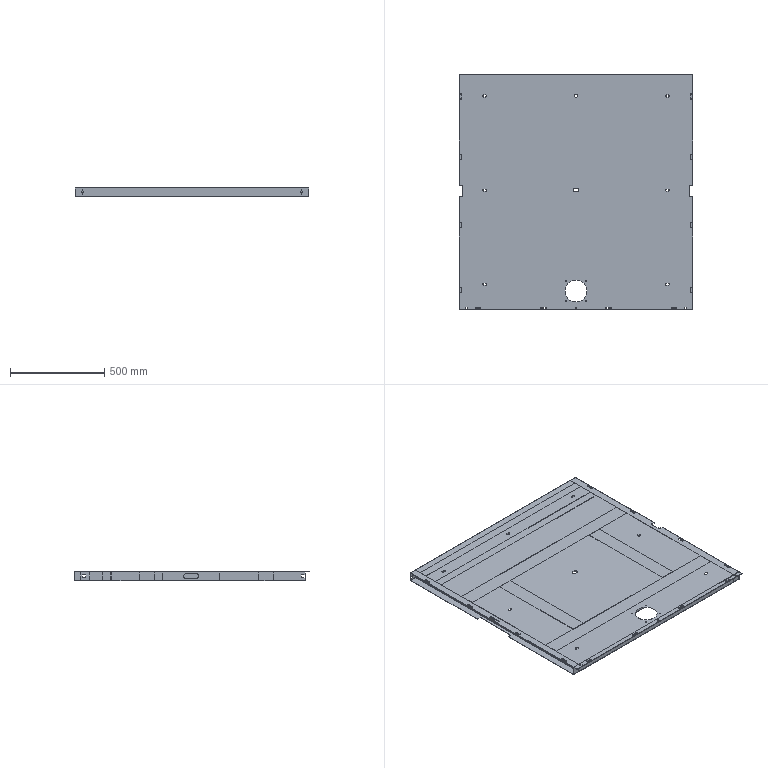Part | 16 solids | 992 faces | box 1240 x 1250 x 49.5 mm | volume 4570648 mm3 | plane 680 | cylinder 288 | cone 24 | commonest cylinder face diameters 10 x76 0.4 x46 3.4 x44 11 x29 20 x27 30 x10